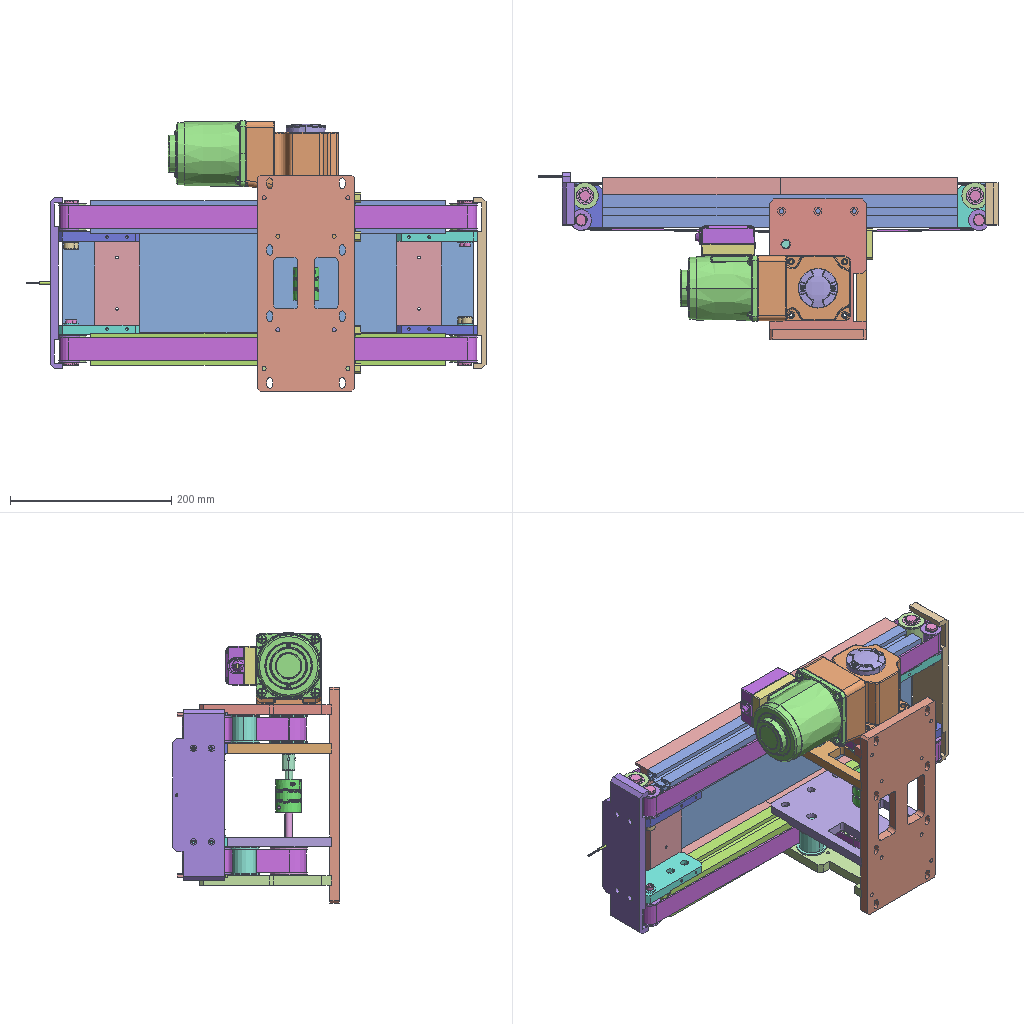Assembly | STEP file | 41 different items | 114 placed | box 571 x 207 x 335 mm
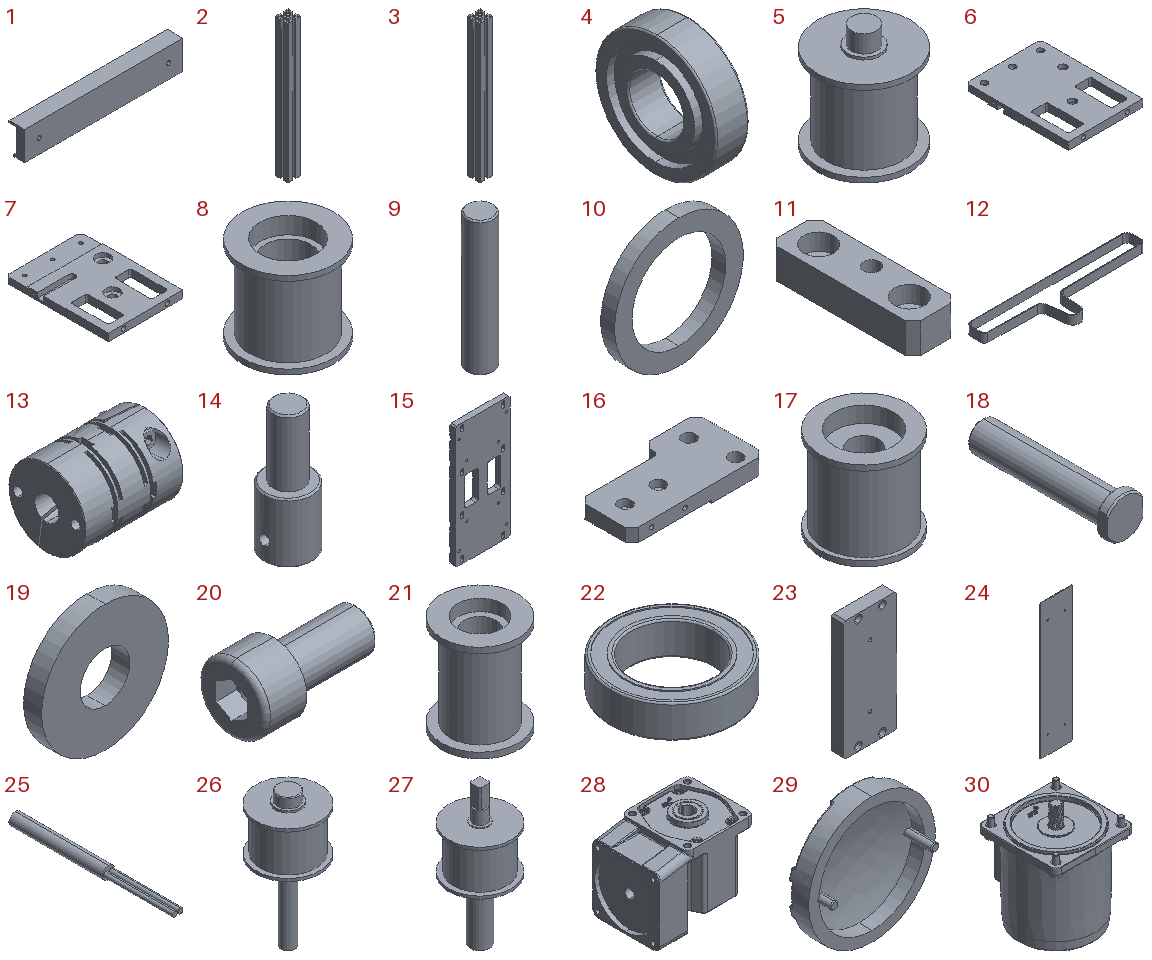Parts list (item | name | quantity | parent item | size | volume):
1 | (PA01.001.LX004) Belt Track | x4 | in Infeed Conveyor Line | 220 x 22 x 40 mm | 130807 mm3
2 | 4040-2 | x1 | in Infeed Conveyor Line | 40 x 40 x 440 mm | 309621 mm3
3 | 4040-1 | x1 | in Infeed Conveyor Line | 40 x 40 x 440 mm | 309621 mm3
4 | B6900ZZ_B6900 | x16 | in Infeed Conveyor Line, Tensioner Pulley, Idler Assembly1, Idler Assembly2 | 6 x 22 x 22 mm | 1551 mm3
5 | (PA01.001.LX015) Idler A | x2 | in Infeed Conveyor Line | 37 x 37 x 50 mm | 26872 mm3
6 | Conveyor Line Bracket-Mirror | x1 | in Infeed Conveyor Line | 120 x 164 x 12 mm | 177189 mm3
7 | (PA01.001.LX002) Conveyor Line Bracket | x1 | in Infeed Conveyor Line | 120 x 164 x 12 mm | 177189 mm3
8 | (PA01.001.LX007) Tensioner Pulley | x2 | in Tensioner Pulley | 36 x 36 x 34 mm | 14967 mm3
9 | (PA01.001.LX008) Tensioner Pulley Shaft | x2 | in Tensioner Pulley | 10 x 10 x 51 mm | 3998 mm3
10 | (PA01.001.LX014) Spacer Ring | x12 | in Tensioner Pulley, Idler Assembly1, Idler Assembly2 | 14 x 1.5 x 14 mm | 108.338 mm3
11 | (PA01.001.LX010) Clamp Block | x4 | in Infeed Conveyor Line | 12 x 38 x 8 mm | 2916 mm3
12 | Belt | x2 | in Infeed Conveyor Line | 518 x 154 x 28 mm | 70875 mm3
13 | MCSLC32_10_10 | x1 | in Infeed Conveyor Line | - | -
14 | (PA01.001.LX009) Connecting Shaft | x1 | in Infeed Conveyor Line | 16 x 16 x 42 mm | 4893 mm3
15 | (PA01.001.LX001) Wheel Train Base Plate | x1 | in Infeed Conveyor Line | 120 x 12 x 268 mm | 319322 mm3
16 | (PA01.001.LX011) Idler Mounting Plate | x2 | in Idler Assembly1 | 100.5 x 52 x 12 mm | 45032 mm3
17 | (PA01.001.LX016) Idler B | x4 | in Idler Assembly1, Idler Assembly2 | 33 x 33 x 33 mm | 17363 mm3
18 | (PA01.001.LX012) Idler Fixed Shaft | x8 | in Idler Assembly1, Idler Assembly2 | 12 x 49 x 14 mm | 3867 mm3
19 | (PA01.001.LX013) Washer | x8 | in Idler Assembly1, Idler Assembly2 | 14 x 2 x 14 mm | 260.359 mm3
20 | hexagon socket head cap screws gb_GB_FASTENER_SCREWS_HSHCS M8X16-N | x4 | in Idler Assembly1 | 24 x 13 x 13 mm | 1715 mm3
21 | (PA01.001.LX017) Idler C | x4 | in Idler Assembly1, Idler Assembly2 | 26 x 26 x 33 mm | 7445 mm3
22 | B6700ZZ_C-B6700ZZ | x8 | in Idler Assembly1, Idler Assembly2 | 15 x 15 x 4 mm | 375.474 mm3
23 | (PA01.001.LX018) Idler Connecting Plate | x2 | in Infeed Conveyor Line | 55 x 13 x 124 mm | 86902 mm3
24 | (PA01.001.LX019) Cover Plate | x1 | in Infeed Conveyor Line | 123 x 2 x 511 mm | 125357 mm3
25 | FU-35FA | x1 | in Infeed Conveyor Line | 3 x 40 x 3 mm | 201.029 mm3
26 | (PA01.001.LX005) Drive Wheel A | x1 | in Infeed Conveyor Line | 46 x 46 x 98 mm | 49218 mm3
27 | (PA01.001.LX006) Drive Wheel B | x1 | in Infeed Conveyor Line | 47 x 47 x 106 mm | 54403 mm3
28 | 80GK-RC | x1 | in 25yt03-180-1 | 115.25 x 80.5 x 92.25 mm | 602584 mm3
29 | FCG-80 | x1 | in 25yt03-180-1 | 49 x 16.126 x 49 mm | 8270 mm3
30 | 80YT25G | x1 | in 80YT25GV22 | 81.679 x 81.24 x 115.2 mm | 124196 mm3
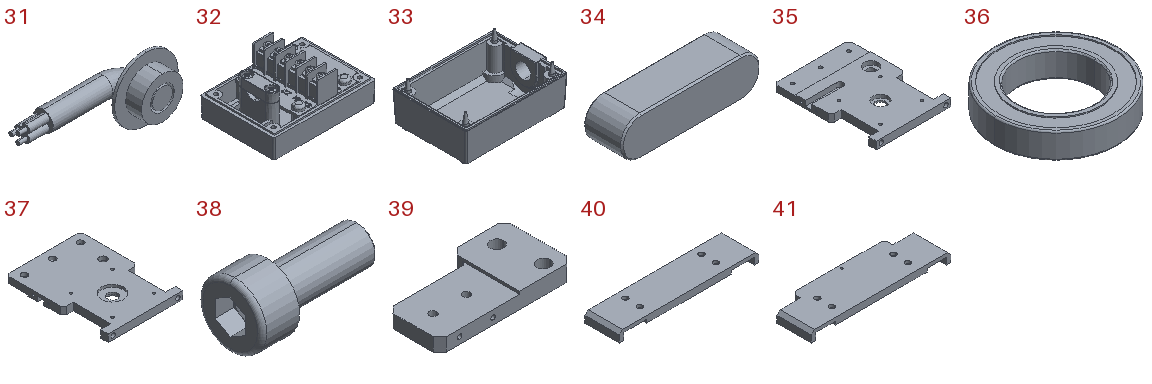31 | YX | x1 | in 80YT25GV22 | 35 x 12.5 x 16 mm | 1115 mm3
32 | JXH-X | x1 | in 80YT25GV22 | 67 x 49 x 34.5 mm | 31444 mm3
33 | JXH-S | x1 | in 80YT25GV22 | 73.93 x 48.93 x 29.5 mm | 22748 mm3
34 | KES5-18 | x1 | in Infeed Conveyor Line | 18 x 5 x 5 mm | 421.523 mm3
35 | (PA01.001.LX003) Motor Mounting Plate | x1 | in Infeed Conveyor Line | 120 x 164 x 12 mm | 186688 mm3
36 | B6802ZZ_C-B6802ZZ | x2 | in Infeed Conveyor Line | 24 x 24 x 5 mm | 1300 mm3
37 | Mirrored Motor Mounting Plate | x1 | in Infeed Conveyor Line | 120 x 164 x 12 mm | 186688 mm3
38 | hexagon socket head cap screws gb_GB_FASTENER_SCREWS_HSHCS M5X12-C | x4 | in Idler Assembly2 | 17 x 8.5 x 8.5 mm | 477.396 mm3
39 | Mirrored Idler Mounting Plate | x2 | in Idler Assembly2 | 100.5 x 52 x 12 mm | 45032 mm3
40 | (PA01.001.LX020) Stop Block A | x1 | in Infeed Conveyor Line | 213 x 52 x 15.5 mm | 94023 mm3
41 | (PA01.001.LX021) Stop Block B | x1 | in Infeed Conveyor Line | 213 x 65 x 15.5 mm | 114748 mm3
Placements (level | parent | child | x y z in mm | rotation matrix by rows):
1 | Infeed Conveyor Line | (PA01.001.LX004) Belt Track | -135.043 -10.927 20.0 | 1 0 0 0 1 0 0 0 1
1 | Infeed Conveyor Line | 4040-2 | 84.957 -30.927 0.0 | 0 0 -1 0 1 0 1 0 0
1 | Infeed Conveyor Line | (PA01.001.LX004) Belt Track | -355.043 -10.927 20.0 | 1 0 0 0 1 0 0 0 1
1 | Infeed Conveyor Line | 4040-1 | 84.957 -30.927 -164.0 | 0 0 -1 0 1 0 1 0 0
1 | Infeed Conveyor Line | (PA01.001.LX004) Belt Track | 84.957 -10.927 -184.0 | -1 0 0 0 1 0 0 0 -1
1 | Infeed Conveyor Line | (PA01.001.LX004) Belt Track | -135.043 -10.927 -184.0 | -1 0 0 0 1 0 0 0 -1
1 | Infeed Conveyor Line | B6900ZZ_B6900 | -128.043 -71.927 18.2 | 0 -0.5138 -0.8579 0 0.8579 -0.5138 1 0 0
1 | Infeed Conveyor Line | (PA01.001.LX015) Idler A | -128.043 -71.927 0.2 | 0.9965 0.0833 0 -0.0833 0.9965 0 0 0 1
1 | Infeed Conveyor Line | Conveyor Line Bracket-Mirror | -88.043 -97.927 -30.0 | -1 0 0 0 1 0 0 0 -1
1 | Infeed Conveyor Line | (PA01.001.LX002) Conveyor Line Bracket | -88.043 -97.927 -134.0 | -1 0 0 0 1 0 0 0 -1
1 | Infeed Conveyor Line | Tensioner Pulley | -46.88 -70.309 -0.1 | 1 0 0 0 1 0 0 0 1
2 | Tensioner Pulley | (PA01.001.LX007) Tensioner Pulley | 2.837 -1.617 -0.0 | 1 0 0 0 1 0 0 0 1
2 | Tensioner Pulley | B6900ZZ_B6900 | 2.837 -1.617 16.4 | 0 0 1 0 1 0 -1 0 0
2 | Tensioner Pulley | B6900ZZ_B6900 | 2.837 -1.617 -16.4 | 0 0 -1 0 1 0 1 0 0
2 | Tensioner Pulley | (PA01.001.LX008) Tensioner Pulley Shaft | 2.837 -1.617 -0.0 | 1 0 0 0 1 0 0 0 1
2 | Tensioner Pulley | (PA01.001.LX014) Spacer Ring | 2.837 -1.617 17.9 | 1 0 0 0 0 1 0 -1 0
2 | Tensioner Pulley | (PA01.001.LX014) Spacer Ring | 2.837 -1.617 -17.9 | 1 0 0 0 0 -1 0 1 0
1 | Infeed Conveyor Line | (PA01.001.LX010) Clamp Block | -28.043 -71.927 24.0 | 0 0 1 0 1 0 -1 0 -0
1 | Infeed Conveyor Line | (PA01.001.LX010) Clamp Block | -28.043 -71.927 -24.0 | 0 0 1 0 -1 0 1 0 0
1 | Infeed Conveyor Line | Belt | -88.043 -126.927 -150.0 | -1 0 0 0 1 0 0 0 -1
1 | Infeed Conveyor Line | B6900ZZ_B6900 | -128.043 -71.927 -140.0 | 0 0 1 0 1 0 -1 0 -0
1 | Infeed Conveyor Line | B6900ZZ_B6900 | -88.043 -126.927 -140.0 | 0 0 1 0 1 0 -1 0 -0
1 | Infeed Conveyor Line | Tensioner Pulley | -40.8 -72.309 -164.0 | -0.9208 0.39 0 -0.39 -0.9208 0 0 0 1
2 | Tensioner Pulley | (PA01.001.LX007) Tensioner Pulley | 2.837 -1.617 -0.0 | 1 0 0 0 1 0 0 0 1
2 | Tensioner Pulley | B6900ZZ_B6900 | 2.837 -1.617 16.4 | 0 0 1 0 1 0 -1 0 0
2 | Tensioner Pulley | B6900ZZ_B6900 | 2.837 -1.617 -16.4 | 0 0 -1 0 1 0 1 0 0
2 | Tensioner Pulley | (PA01.001.LX008) Tensioner Pulley Shaft | 2.837 -1.617 -0.0 | 1 0 0 0 1 0 0 0 1
2 | Tensioner Pulley | (PA01.001.LX014) Spacer Ring | 2.837 -1.617 17.9 | 1 0 0 0 0 1 0 -1 0
2 | Tensioner Pulley | (PA01.001.LX014) Spacer Ring | 2.837 -1.617 -17.9 | 1 0 0 0 0 -1 0 1 0
1 | Infeed Conveyor Line | (PA01.001.LX015) Idler A | -128.043 -71.927 -164.0 | -0.04633 -0.9989 0 -0.9989 0.04633 0 0 0 -1
1 | Infeed Conveyor Line | MCSLC32_10_10 | -88.043 -126.927 -62.372 | 0 -0.9659 0.259 0 0.259 0.9659 -1 0 0
1 | Infeed Conveyor Line | (PA01.001.LX009) Connecting Shaft | -88.043 -126.927 -30.838 | 1 0 0 0 -1 0 0 0 -1
1 | Infeed Conveyor Line | (PA01.001.LX001) Wheel Train Base Plate | -148.043 -189.927 52.0 | 1 0 0 0 1 0 0 0 1
1 | Infeed Conveyor Line | B6900ZZ_B6900 | -103.043 -81.927 -188.0 | 0 -0.7036 -0.7105 0 0.7105 -0.7036 1 0 0
1 | Infeed Conveyor Line | Idler Assembly1 | -80.0 0.0 -164.0 | 1 0 0 0 1 0 0 0 1
2 | Idler Assembly1 | (PA01.001.LX011) Idler Mounting Plate | 104.957 -50.927 20.0 | 1 0 0 0 1 0 0 0 1
2 | Idler Assembly1 | (PA01.001.LX016) Idler B | 186.957 -11.927 -0.0 | 1 0 0 0 1 0 0 0 1
2 | Idler Assembly1 | B6900ZZ_B6900 | 186.957 -11.927 16.5 | 0 0.3431 0.9393 0 0.9393 -0.3431 -1 0 0
2 | Idler Assembly1 | B6900ZZ_B6900 | 186.957 -11.927 -16.5 | 0 0 -1 0 1 0 1 0 0
2 | Idler Assembly1 | (PA01.001.LX012) Idler Fixed Shaft | 186.957 -11.927 -20.0 | -0.4698 0 -0.8828 -0.8828 0 0.4698 0 1 0
2 | Idler Assembly1 | (PA01.001.LX014) Spacer Ring | 186.957 -11.927 16.5 | 1 0 0 0 0 -1 0 1 0
2 | Idler Assembly1 | (PA01.001.LX014) Spacer Ring | 191.957 -41.927 16.5 | 1 0 0 0 0 -1 0 1 0
2 | Idler Assembly1 | (PA01.001.LX012) Idler Fixed Shaft | 191.957 -41.927 -20.0 | 1 0 0 0 0 -1 0 1 0
2 | Idler Assembly1 | (PA01.001.LX013) Washer | 186.957 -11.927 32.0 | 1 0 0 0 0 1 0 -1 0
2 | Idler Assembly1 | (PA01.001.LX013) Washer | 191.957 -41.927 32.0 | 1 0 0 0 0 1 0 -1 0
2 | Idler Assembly1 | hexagon socket head cap screws gb_GB_FASTENER_SCREWS_HSHCS M8X16-N | 186.957 -11.927 40.0 | 0 0 1 0 1 0 -1 0 0
2 | Idler Assembly1 | hexagon socket head cap screws gb_GB_FASTENER_SCREWS_HSHCS M8X16-N | 191.957 -41.927 40.0 | 0 0 1 0 1 0 -1 0 0
2 | Idler Assembly1 | (PA01.001.LX017) Idler C | 191.957 -41.927 -0.0 | 0.8788 -0.4771 0 0.4771 0.8788 0 0 0 1
2 | Idler Assembly1 | B6700ZZ_C-B6700ZZ | 191.957 -41.927 16.5 | 1 0 0 0 1 0 0 0 1
2 | Idler Assembly1 | B6700ZZ_C-B6700ZZ | 191.957 -41.927 -12.5 | 1 0 0 0 1 0 0 0 1
1 | Infeed Conveyor Line | Idler Assembly1 | -190.086 0.0 -0.0 | -1 0 0 0 1 0 0 0 -1
2 | Idler Assembly1 | (PA01.001.LX011) Idler Mounting Plate | 104.957 -50.927 20.0 | 1 0 0 0 1 0 0 0 1
2 | Idler Assembly1 | (PA01.001.LX016) Idler B | 186.957 -11.927 -0.0 | 1 0 0 0 1 0 0 0 1
2 | Idler Assembly1 | B6900ZZ_B6900 | 186.957 -11.927 16.5 | 0 0.3431 0.9393 0 0.9393 -0.3431 -1 0 0
2 | Idler Assembly1 | B6900ZZ_B6900 | 186.957 -11.927 -16.5 | 0 0 -1 0 1 0 1 0 0
2 | Idler Assembly1 | (PA01.001.LX012) Idler Fixed Shaft | 186.957 -11.927 -20.0 | -0.4698 0 -0.8828 -0.8828 0 0.4698 0 1 0
2 | Idler Assembly1 | (PA01.001.LX014) Spacer Ring | 186.957 -11.927 16.5 | 1 0 0 0 0 -1 0 1 0
2 | Idler Assembly1 | (PA01.001.LX014) Spacer Ring | 191.957 -41.927 16.5 | 1 0 0 0 0 -1 0 1 0
2 | Idler Assembly1 | (PA01.001.LX012) Idler Fixed Shaft | 191.957 -41.927 -20.0 | 1 0 0 0 0 -1 0 1 0
2 | Idler Assembly1 | (PA01.001.LX013) Washer | 186.957 -11.927 32.0 | 1 0 0 0 0 1 0 -1 0
2 | Idler Assembly1 | (PA01.001.LX013) Washer | 191.957 -41.927 32.0 | 1 0 0 0 0 1 0 -1 0
2 | Idler Assembly1 | hexagon socket head cap screws gb_GB_FASTENER_SCREWS_HSHCS M8X16-N | 186.957 -11.927 40.0 | 0 0 1 0 1 0 -1 0 0
2 | Idler Assembly1 | hexagon socket head cap screws gb_GB_FASTENER_SCREWS_HSHCS M8X16-N | 191.957 -41.927 40.0 | 0 0 1 0 1 0 -1 0 0
2 | Idler Assembly1 | (PA01.001.LX017) Idler C | 191.957 -41.927 -0.0 | 0.8788 -0.4771 0 0.4771 0.8788 0 0 0 1
2 | Idler Assembly1 | B6700ZZ_C-B6700ZZ | 191.957 -41.927 16.5 | 1 0 0 0 1 0 0 0 1
2 | Idler Assembly1 | B6700ZZ_C-B6700ZZ | 191.957 -41.927 -12.5 | 1 0 0 0 1 0 0 0 1
1 | Infeed Conveyor Line | (PA01.001.LX018) Idler Connecting Plate | 79.957 2.073 -20.0 | -1 0 0 0 -1 0 0 0 1
1 | Infeed Conveyor Line | (PA01.001.LX018) Idler Connecting Plate | -295.043 2.073 -20.0 | -1 0 0 0 -1 0 0 0 1
1 | Infeed Conveyor Line | (PA01.001.LX019) Cover Plate | -390.543 4.073 -20.5 | 0 0 1 0 1 0 -1 0 -0
1 | Infeed Conveyor Line | FU-35FA | -418.543 12.073 -82.0 | 0 1 0 -1 0 0 0 0 1
1 | Infeed Conveyor Line | (PA01.001.LX010) Clamp Block | -28.043 -71.927 -140.0 | 0 0 1 0 1 0 -1 0 -0
1 | Infeed Conveyor Line | (PA01.001.LX010) Clamp Block | -28.043 -71.927 -188.0 | 0 0 1 0 -1 0 1 0 0
1 | Infeed Conveyor Line | (PA01.001.LX005) Drive Wheel A | -88.043 -126.927 -164.0 | -0.6557 0.7551 0 0.7551 0.6557 0 0 0 -1
1 | Infeed Conveyor Line | (PA01.001.LX006) Drive Wheel B | -88.043 -126.927 0.0 | 1 0 0 0 -1 0 0 0 -1
1 | Infeed Conveyor Line | 25yt03-180-1 | -163.043 -126.927 78.5 | 1 0 0 0 -1 0 0 0 -1
2 | 25yt03-180-1 | 80GK-RC | 75.0 -0.0 48.5 | 1 0 0 0 1 0 0 0 1
2 | 25yt03-180-1 | FCG-80 | 75.0 -0.0 -26.5 | 1 0 0 0 0 1 0 -1 0
2 | 25yt03-180-1 | 80YT25GV22 | -0.0 -0.0 0.0 | 1 0 0 0 -1 0 0 0 -1
3 | 80YT25GV22 | 80YT25G | -0.0 -0.0 -0.0 | 0 0 1 0 1 0 -1 0 -0
3 | 80YT25GV22 | YX | -13.0 42.4 -0.0 | 1 0 0 0 1 0 0 0 1
3 | 80YT25GV22 | JXH-X | -36.5 41.4 -0.0 | 1 0 0 0 0 1 0 -1 -0
3 | 80YT25GV22 | JXH-S | -36.5 78.4 0.0 | -1 0 0 0 0 -1 0 -1 0
1 | Infeed Conveyor Line | KES5-18 | -88.043 -136.427 48.5 | 0 0 1 0 1 0 -1 0 0
1 | Infeed Conveyor Line | (PA01.001.LX003) Motor Mounting Plate | -88.043 -97.927 30.0 | -1 0 0 0 1 0 0 0 -1
1 | Infeed Conveyor Line | B6802ZZ_C-B6802ZZ | -88.043 -126.927 23.2 | 1 0 0 0 1 0 0 0 1
1 | Infeed Conveyor Line | B6802ZZ_C-B6802ZZ | -88.043 -126.927 -182.0 | 1 0 0 0 1 0 0 0 1
1 | Infeed Conveyor Line | Mirrored Motor Mounting Plate | -88.043 -97.927 -194.0 | -1 0 0 0 1 0 0 0 -1
1 | Infeed Conveyor Line | Belt | -88.043 -126.927 14.0 | -1 0 0 0 1 0 0 0 -1
1 | Infeed Conveyor Line | Idler Assembly2 | -112.989 7.313 25.404 | 1 0 0 0 1 0 0 0 1
2 | Idler Assembly2 | (PA01.001.LX016) Idler B | 219.946 -19.24 -25.404 | -0.9237 -0.383 0 -0.383 0.9237 0 0 0 -1
2 | Idler Assembly2 | B6900ZZ_B6900 | 219.946 -19.24 -41.904 | 0 -0.6767 -0.7363 0 0.7363 -0.6767 1 0 0
2 | Idler Assembly2 | B6900ZZ_B6900 | 219.946 -19.24 -8.904 | 0 -0.383 0.9237 0 0.9237 0.383 -1 0 0
2 | Idler Assembly2 | (PA01.001.LX012) Idler Fixed Shaft | 219.946 -19.24 -5.404 | 0.7721 0 0.6355 -0.6355 0 0.7721 0 -1 0
2 | Idler Assembly2 | (PA01.001.LX014) Spacer Ring | 219.946 -19.24 -41.904 | -0.9237 0 0.383 -0.383 0 -0.9237 0 -1 0
2 | Idler Assembly2 | (PA01.001.LX014) Spacer Ring | 224.946 -49.24 -41.904 | -0.9237 0 0.383 -0.383 0 -0.9237 0 -1 0
2 | Idler Assembly2 | (PA01.001.LX012) Idler Fixed Shaft | 224.946 -49.24 -5.404 | -0.9237 0 0.383 -0.383 0 -0.9237 0 -1 0
2 | Idler Assembly2 | (PA01.001.LX013) Washer | 219.946 -19.24 -57.404 | -0.9996 0 0.02817 0.02817 0 0.9996 0 1 0
2 | Idler Assembly2 | (PA01.001.LX013) Washer | 224.946 -49.24 -57.404 | -0.9237 0 -0.383 -0.383 0 0.9237 0 1 0
2 | Idler Assembly2 | hexagon socket head cap screws gb_GB_FASTENER_SCREWS_HSHCS M5X12-C | 219.946 -19.24 -62.404 | 0 -0.383 -0.9237 0 0.9237 -0.383 1 0 0
2 | Idler Assembly2 | hexagon socket head cap screws gb_GB_FASTENER_SCREWS_HSHCS M5X12-C | 224.946 -49.24 -62.404 | 0 -0.383 -0.9237 0 0.9237 -0.383 1 0 0
2 | Idler Assembly2 | (PA01.001.LX017) Idler C | 224.946 -49.24 -25.404 | -0.7012 -0.713 0 -0.713 0.7012 0 0 0 -1
2 | Idler Assembly2 | B6700ZZ_C-B6700ZZ | 224.946 -49.24 -41.904 | -0.9237 -0.383 0 -0.383 0.9237 0 0 0 -1
2 | Idler Assembly2 | B6700ZZ_C-B6700ZZ | 224.946 -49.24 -12.904 | -0.9237 -0.383 0 -0.383 0.9237 0 0 0 -1
2 | Idler Assembly2 | Mirrored Idler Mounting Plate | 137.946 -58.24 -45.404 | 1 0 0 0 1 0 0 0 1
1 | Infeed Conveyor Line | Idler Assembly2 | -157.097 7.313 -189.404 | -1 0 0 0 1 0 0 0 -1
2 | Idler Assembly2 | (PA01.001.LX016) Idler B | 219.946 -19.24 -25.404 | -0.9237 -0.383 0 -0.383 0.9237 0 0 0 -1
2 | Idler Assembly2 | B6900ZZ_B6900 | 219.946 -19.24 -41.904 | 0 -0.6767 -0.7363 0 0.7363 -0.6767 1 0 0
2 | Idler Assembly2 | B6900ZZ_B6900 | 219.946 -19.24 -8.904 | 0 -0.383 0.9237 0 0.9237 0.383 -1 0 0
2 | Idler Assembly2 | (PA01.001.LX012) Idler Fixed Shaft | 219.946 -19.24 -5.404 | 0.7721 0 0.6355 -0.6355 0 0.7721 0 -1 0
2 | Idler Assembly2 | (PA01.001.LX014) Spacer Ring | 219.946 -19.24 -41.904 | -0.9237 0 0.383 -0.383 0 -0.9237 0 -1 0
2 | Idler Assembly2 | (PA01.001.LX014) Spacer Ring | 224.946 -49.24 -41.904 | -0.9237 0 0.383 -0.383 0 -0.9237 0 -1 0
2 | Idler Assembly2 | (PA01.001.LX012) Idler Fixed Shaft | 224.946 -49.24 -5.404 | -0.9237 0 0.383 -0.383 0 -0.9237 0 -1 0
2 | Idler Assembly2 | (PA01.001.LX013) Washer | 219.946 -19.24 -57.404 | -0.9996 0 0.02817 0.02817 0 0.9996 0 1 0
2 | Idler Assembly2 | (PA01.001.LX013) Washer | 224.946 -49.24 -57.404 | -0.9237 0 -0.383 -0.383 0 0.9237 0 1 0
2 | Idler Assembly2 | hexagon socket head cap screws gb_GB_FASTENER_SCREWS_HSHCS M5X12-C | 219.946 -19.24 -62.404 | 0 -0.383 -0.9237 0 0.9237 -0.383 1 0 0
2 | Idler Assembly2 | hexagon socket head cap screws gb_GB_FASTENER_SCREWS_HSHCS M5X12-C | 224.946 -49.24 -62.404 | 0 -0.383 -0.9237 0 0.9237 -0.383 1 0 0
2 | Idler Assembly2 | (PA01.001.LX017) Idler C | 224.946 -49.24 -25.404 | -0.7012 -0.713 0 -0.713 0.7012 0 0 0 -1
2 | Idler Assembly2 | B6700ZZ_C-B6700ZZ | 224.946 -49.24 -41.904 | -0.9237 -0.383 0 -0.383 0.9237 0 0 0 -1
2 | Idler Assembly2 | B6700ZZ_C-B6700ZZ | 224.946 -49.24 -12.904 | -0.9237 -0.383 0 -0.383 0.9237 0 0 0 -1
2 | Idler Assembly2 | Mirrored Idler Mounting Plate | 137.946 -58.24 -45.404 | 1 0 0 0 1 0 0 0 1
1 | Infeed Conveyor Line | (PA01.001.LX020) Stop Block A | 135.457 -65.927 -82.0 | 0 0 1 0 1 0 -1 0 0
1 | Infeed Conveyor Line | (PA01.001.LX021) Stop Block B | -405.543 -65.927 -82.0 | 0 0 -1 0 1 0 1 0 0